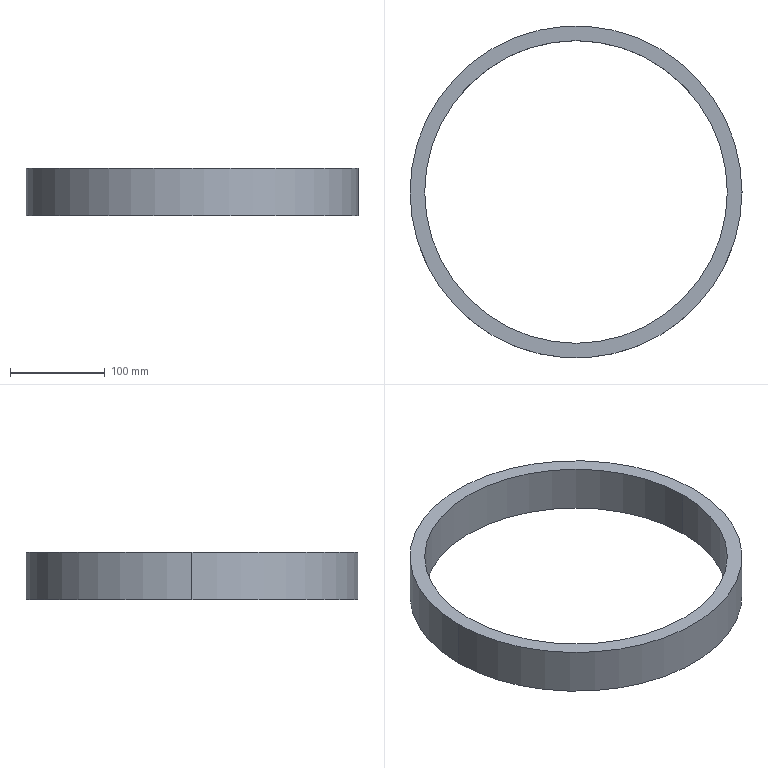Part | SolidWorks | features Extrusion 1 | 1 solid | 6 faces | box 350 x 350 x 50 mm | volume 814419 mm3 | cylinder 4 | plane 2 | commonest cylinder face diameters 319 x2 350 x2
STEP:
#1=CARTESIAN_POINT('',(-159.5,0.,25.));
#2=VERTEX_POINT('',#1);
#3=CARTESIAN_POINT('',(159.5,0.,25.));
#4=VERTEX_POINT('',#3);
#5=CARTESIAN_POINT('',(0.,0.,25.));
#6=DIRECTION('',(0.,0.,1.));
#7=DIRECTION('',(1.,0.,0.));
#8=AXIS2_PLACEMENT_3D('',#5,#6,#7);
#9=CIRCLE('',#8,159.5);
#10=EDGE_CURVE('',#2,#4,#9,.T.);
#11=ORIENTED_EDGE('',*,*,#10,.T.);
#12=CARTESIAN_POINT('',(159.5,0.,-25.));
#13=VERTEX_POINT('',#12);
#14=CARTESIAN_POINT('',(159.5,0.,25.));
#15=DIRECTION('',(0.,0.,-1.));
#16=VECTOR('',#15,1000.);
#17=LINE('',#14,#16);
#18=EDGE_CURVE('',#4,#13,#17,.T.);
#19=ORIENTED_EDGE('',*,*,#18,.T.);
#20=CARTESIAN_POINT('',(-159.5,0.,-25.));
#21=VERTEX_POINT('',#20);
#22=CARTESIAN_POINT('',(0.,0.,-25.));
#23=DIRECTION('',(0.,0.,1.));
#24=DIRECTION('',(1.,0.,0.));
#25=AXIS2_PLACEMENT_3D('',#22,#23,#24);
#26=CIRCLE('',#25,159.5);
#27=EDGE_CURVE('',#21,#13,#26,.T.);
#28=ORIENTED_EDGE('',*,*,#27,.F.);
#29=CARTESIAN_POINT('',(-159.5,0.,25.));
#30=DIRECTION('',(0.,0.,-1.));
#31=VECTOR('',#30,1000.);
#32=LINE('',#29,#31);
#33=EDGE_CURVE('',#2,#21,#32,.T.);
#34=ORIENTED_EDGE('',*,*,#33,.F.);
#35=EDGE_LOOP('',(#11,#19,#28,#34));
#36=FACE_OUTER_BOUND('',#35,.T.);
#37=CARTESIAN_POINT('',(0.,0.,25.));
#38=DIRECTION('',(0.,0.,-1.));
#39=DIRECTION('',(-1.,0.,0.));
#40=AXIS2_PLACEMENT_3D('',#37,#38,#39);
#41=CYLINDRICAL_SURFACE('',#40,159.5);
#42=ADVANCED_FACE('',(#36),#41,.F.);
#43=CARTESIAN_POINT('',(175.,0.,25.));
#44=VERTEX_POINT('',#43);
#45=CARTESIAN_POINT('',(-175.,0.,25.));
#46=VERTEX_POINT('',#45);
#47=CARTESIAN_POINT('',(0.,0.,25.));
#48=DIRECTION('',(0.,0.,1.));
#49=DIRECTION('',(1.,0.,0.));
#50=AXIS2_PLACEMENT_3D('',#47,#48,#49);
#51=CIRCLE('',#50,175.);
#52=EDGE_CURVE('',#44,#46,#51,.T.);
#53=ORIENTED_EDGE('',*,*,#52,.F.);
#54=CARTESIAN_POINT('',(175.,0.,-25.));
#55=VERTEX_POINT('',#54);
#56=CARTESIAN_POINT('',(175.,0.,25.));
#57=DIRECTION('',(0.,0.,-1.));
#58=VECTOR('',#57,1000.);
#59=LINE('',#56,#58);
#60=EDGE_CURVE('',#44,#55,#59,.T.);
#61=ORIENTED_EDGE('',*,*,#60,.T.);
#62=CARTESIAN_POINT('',(-175.,0.,-25.));
#63=VERTEX_POINT('',#62);
#64=CARTESIAN_POINT('',(0.,0.,-25.));
#65=DIRECTION('',(0.,0.,1.));
#66=DIRECTION('',(1.,0.,0.));
#67=AXIS2_PLACEMENT_3D('',#64,#65,#66);
#68=CIRCLE('',#67,175.);
#69=EDGE_CURVE('',#55,#63,#68,.T.);
#70=ORIENTED_EDGE('',*,*,#69,.T.);
#71=CARTESIAN_POINT('',(-175.,0.,25.));
#72=DIRECTION('',(0.,0.,-1.));
#73=VECTOR('',#72,1000.);
#74=LINE('',#71,#73);
#75=EDGE_CURVE('',#46,#63,#74,.T.);
#76=ORIENTED_EDGE('',*,*,#75,.F.);
#77=EDGE_LOOP('',(#53,#61,#70,#76));
#78=FACE_OUTER_BOUND('',#77,.T.);
#79=CARTESIAN_POINT('',(0.,0.,25.));
#80=DIRECTION('',(0.,0.,-1.));
#81=DIRECTION('',(-1.,0.,0.));
#82=AXIS2_PLACEMENT_3D('',#79,#80,#81);
#83=CYLINDRICAL_SURFACE('',#82,175.);
#84=ADVANCED_FACE('',(#78),#83,.T.);
#85=CARTESIAN_POINT('',(0.,0.,25.));
#86=DIRECTION('',(0.,0.,1.));
#87=DIRECTION('',(1.,0.,0.));
#88=AXIS2_PLACEMENT_3D('',#85,#86,#87);
#89=CIRCLE('',#88,175.);
#90=EDGE_CURVE('',#46,#44,#89,.T.);
#91=ORIENTED_EDGE('',*,*,#90,.T.);
#92=ORIENTED_EDGE('',*,*,#52,.T.);
#93=EDGE_LOOP('',(#91,#92));
#94=FACE_OUTER_BOUND('',#93,.T.);
#95=ORIENTED_EDGE('',*,*,#10,.F.);
#96=CARTESIAN_POINT('',(0.,0.,25.));
#97=DIRECTION('',(0.,0.,1.));
#98=DIRECTION('',(1.,0.,0.));
#99=AXIS2_PLACEMENT_3D('',#96,#97,#98);
#100=CIRCLE('',#99,159.5);
#101=EDGE_CURVE('',#4,#2,#100,.T.);
#102=ORIENTED_EDGE('',*,*,#101,.F.);
#103=EDGE_LOOP('',(#95,#102));
#104=FACE_BOUND('',#103,.T.);
#105=CARTESIAN_POINT('',(0.,0.,25.));
#106=DIRECTION('',(0.,0.,1.));
#107=DIRECTION('',(1.,0.,0.));
#108=AXIS2_PLACEMENT_3D('',#105,#106,#107);
#109=PLANE('',#108);
#110=ADVANCED_FACE('',(#94,#104),#109,.T.);
#111=CARTESIAN_POINT('',(0.,0.,-25.));
#112=DIRECTION('',(0.,0.,1.));
#113=DIRECTION('',(1.,0.,0.));
#114=AXIS2_PLACEMENT_3D('',#111,#112,#113);
#115=CIRCLE('',#114,175.);
#116=EDGE_CURVE('',#63,#55,#115,.T.);
#117=ORIENTED_EDGE('',*,*,#116,.F.);
#118=ORIENTED_EDGE('',*,*,#69,.F.);
#119=EDGE_LOOP('',(#117,#118));
#120=FACE_OUTER_BOUND('',#119,.T.);
#121=ORIENTED_EDGE('',*,*,#27,.T.);
#122=CARTESIAN_POINT('',(0.,0.,-25.));
#123=DIRECTION('',(0.,0.,1.));
#124=DIRECTION('',(1.,0.,0.));
#125=AXIS2_PLACEMENT_3D('',#122,#123,#124);
#126=CIRCLE('',#125,159.5);
#127=EDGE_CURVE('',#13,#21,#126,.T.);
#128=ORIENTED_EDGE('',*,*,#127,.T.);
#129=EDGE_LOOP('',(#121,#128));
#130=FACE_BOUND('',#129,.T.);
#131=CARTESIAN_POINT('',(0.,0.,-25.));
#132=DIRECTION('',(0.,0.,1.));
#133=DIRECTION('',(1.,0.,0.));
#134=AXIS2_PLACEMENT_3D('',#131,#132,#133);
#135=PLANE('',#134);
#136=ADVANCED_FACE('',(#120,#130),#135,.F.);
#137=ORIENTED_EDGE('',*,*,#60,.F.);
#138=ORIENTED_EDGE('',*,*,#90,.F.);
#139=ORIENTED_EDGE('',*,*,#75,.T.);
#140=ORIENTED_EDGE('',*,*,#116,.T.);
#141=EDGE_LOOP('',(#137,#138,#139,#140));
#142=FACE_OUTER_BOUND('',#141,.T.);
#143=CARTESIAN_POINT('',(0.,0.,25.));
#144=DIRECTION('',(0.,0.,-1.));
#145=DIRECTION('',(-1.,0.,0.));
#146=AXIS2_PLACEMENT_3D('',#143,#144,#145);
#147=CYLINDRICAL_SURFACE('',#146,175.);
#148=ADVANCED_FACE('',(#142),#147,.T.);
#149=ORIENTED_EDGE('',*,*,#18,.F.);
#150=ORIENTED_EDGE('',*,*,#101,.T.);
#151=ORIENTED_EDGE('',*,*,#33,.T.);
#152=ORIENTED_EDGE('',*,*,#127,.F.);
#153=EDGE_LOOP('',(#149,#150,#151,#152));
#154=FACE_OUTER_BOUND('',#153,.T.);
#155=CARTESIAN_POINT('',(0.,0.,25.));
#156=DIRECTION('',(0.,0.,-1.));
#157=DIRECTION('',(-1.,0.,0.));
#158=AXIS2_PLACEMENT_3D('',#155,#156,#157);
#159=CYLINDRICAL_SURFACE('',#158,159.5);
#160=ADVANCED_FACE('',(#154),#159,.F.);
#161=CLOSED_SHELL('',(#42,#84,#110,#136,#148,#160));
#162=MANIFOLD_SOLID_BREP('',#161);
#163=CARTESIAN_POINT('',(0.,0.,0.));
#164=DIRECTION('',(0.,0.,1.));
#165=DIRECTION('',(1.,0.,0.));
#166=AXIS2_PLACEMENT_3D('',#163,#164,#165);
#167=(LENGTH_UNIT()NAMED_UNIT(*)SI_UNIT(.MILLI.,.METRE.));
#168=UNCERTAINTY_MEASURE_WITH_UNIT(LENGTH_MEASURE(0.00001),#167,'','');
#169=(NAMED_UNIT(*)PLANE_ANGLE_UNIT()SI_UNIT($,.RADIAN.));
#170=(NAMED_UNIT(*)SI_UNIT($,.STERADIAN.)SOLID_ANGLE_UNIT());
#171=(GEOMETRIC_REPRESENTATION_CONTEXT(3)GLOBAL_UNCERTAINTY_ASSIGNED_CONTEXT((#168))GLOBAL_UNIT_ASSIGNED_CONTEXT((#167,#169,#170))REPRESENTATION_CONTEXT('',''));
#172=ADVANCED_BREP_SHAPE_REPRESENTATION('',(#162,#166),#171);